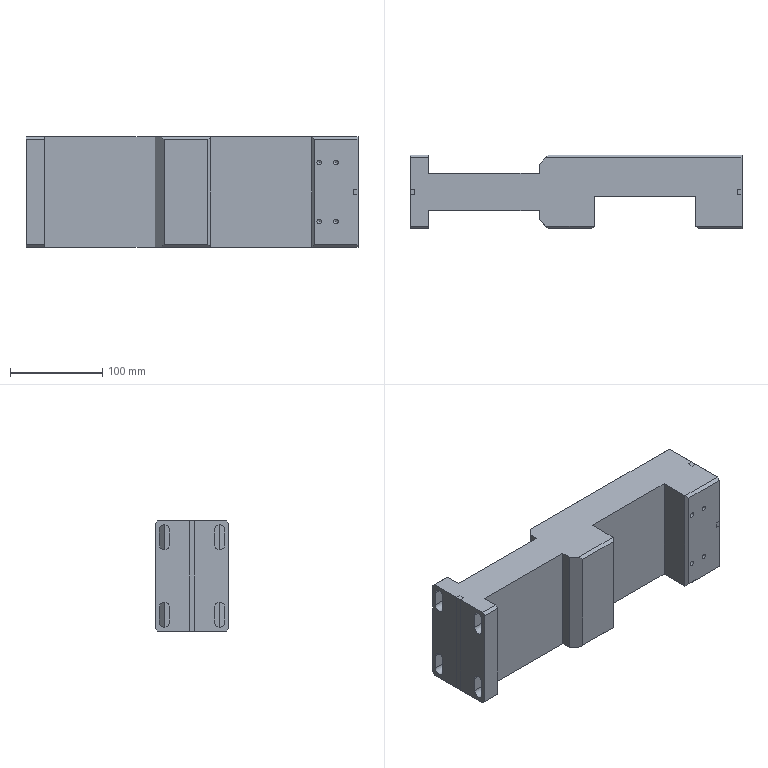CAM job | NX | 3+2 milling, drilling | part box 360 x 80 x 120 mm | stock box 365 x 85 x 125 mm
Tools:
number,name,description,diameter,corner_radius,flute_length,length,flutes
4,D4,平底铣刀-粗,4.0,0.0,25.0,75.0,2
6,D6,平底铣刀-粗,6.0,0.0,25.0,75.0,2
9,D10,平底铣刀-粗,10.0,0.0,35.0,75.0,2
23,D16,平底铣刀-粗,16.0,0.0,50.0,75.0,2
11,D4-J,平底铣刀-精,4.0,0.0,50.0,75.0,2
7,D6-J,平底铣刀-精,6.0,0.0,25.0,75.0,2
10,D10-J,平底铣刀-精,10.0,0.0,35.0,75.0,2
24,D16-J,平底铣刀-精,16.0,0.0,50.0,75.0,2
17,D6R0.5,圆鼻刀-粗,6.0,0.5,50.0,75.0,2
1,D80R0.8飞刀,圆鼻刀-粗,80.0,0.8,50.0,75.0,2
1,D80R0.8飞刀-J,圆鼻刀-精,80.0,0.8,50.0,75.0,2
2,D6倒角刀,倒角刀,6.0,0.0,3.0,25.0,2
18,M6X1.0,丝锥,5.0,0.0,35.0,50.0,2
17,M8X1.25,丝锥,6.8,0.0,35.0,50.0,2
15,ZT5.1,钻头,5.1,0.0,35.0,50.0,2
16,ZT6.9,Drilling Tool,6.9,0.0,35.0,50.0,2
Operations:
program,operation,operation_type,tool,method,geometry_group,spindle_rpm,surface_speed,feed_per_tooth,feed_cut,feed_plunge,cut_length_mm,path_length_mm,cut_time_min,machine_time_min
A,顶面,FaceMilling,D80R0.8飞刀,侧刃精光-切深K-步距G,W-A,4500.0,1385.0,0.1667,1500.0,100.0,1434.0,1530.0,0.956,0.9656
A,打点-深0.8,Operation,D6倒角刀,NONE,W-A,8000.0,150.796,0.0312,500.0,90.0,7.2,217.463,0.0144,0.0354
A,NG_盲锥孔-M6螺纹底孔,Operation,ZT5.1,NONE,W-A,2500.0,39.27,0.03,150.0,90.0,80.0,363.063,0.5333,0.5616
A,外形粗_2,VolumeBased25DMillingOperation,D16,METHOD,W-A,6000.0,301.593,0.5,6000.0,80.0,103112.699,103291.199,17.185,17.203
A,底壁粗_1,VolumeBased25DMillingOperation,D10,METHOD,W-A,9000.0,282.743,0.3333,6000.0,100.0,90760.242,93048.363,15.127,15.355
A,型腔铣开粗-中_COPY,CavityMilling,D10,分层开粗-切深K-步距G,W-A,8000.0,251.32,0.25,4000.0,100.0,7408.75,7808.48,1.852,1.907
A,型腔铣开粗-中_COPY_COPY,CavityMilling,D10,分层开粗-切深K-步距G,W-A,8000.0,251.32,0.25,4000.0,100.0,6245.453,7228.488,1.561,1.694
A,仅选体,SurfaceContour,D6倒角刀,METHOD,W-A,8000.0,150.796,0.1875,3000.0,100.0,673.495,1903.981,0.2245,0.3475
A,铣倒角_1,PlanarMilling,D6倒角刀,METHOD,W-A,8000.0,150.796,0.0375,600.0,100.0,75.821,582.245,0.1264,0.177
A,等高精光往复爬面_COPY,ZLevelMilling,D6R0.5,等高爬面-切深K-步距G,W-A,8000.0,150.796,0.25,4000.0,100.0,18105.798,18137.444,4.526,4.53
A,等高精光往复爬面_COPY_COPY,ZLevelMilling,D6R0.5,等高爬面-切深K-步距G,W-A,8000.0,150.796,0.25,4000.0,100.0,23657.928,24279.462,5.915,5.977
A,底精_1,VolumeBased25DMillingOperation,D10-J,METHOD,W-A,9000.0,169.646,0.0833,1500.0,100.0,2237.2,2376.2,1.492,1.505
A,底侧精_3,VolumeBased25DMillingOperation,D10-J,METHOD,W-A,9000.0,169.646,0.0833,1500.0,100.0,800.05,2139.41,0.5334,0.6673
A,盲锥孔-攻牙M6,Operation,M6X1.0,METHOD,W-A,500.0,7.854,0.001,1.0,90.0,64.0,331.063,64.0,64.027
A,外形半精_2,VolumeBased25DMillingOperation,D16-J,METHOD,W-A,5000.0,251.327,0.12,1200.0,100.0,7106.76,8454.822,5.922,6.057
B,底壁铣飞面开粗_COPY,VolumeBased25DMillingOperation,D80R0.8飞刀,分层开粗-切深K-步距G,W-B,2800.0,703.696,0.5357,3000.0,100.0,8697.187,9307.757,2.899,2.96
B,底壁铣飞面精光_COPY,VolumeBased25DMillingOperation,D80R0.8飞刀-J,侧刃精光-切深K-步距G,W-B,4000.0,1005.28,0.125,1000.0,100.0,1399.584,1495.584,1.4,1.409
B,型腔铣开粗-中_COPY_1,CavityMilling,D10,分层开粗-切深K-步距G,W-B,8000.0,251.32,0.25,4000.0,100.0,167817.825,175313.691,41.955,43.014
B,打点-深0.8_2,Operation,D6倒角刀,NONE,W-B,8000.0,150.796,0.0312,500.0,90.0,7.2,217.463,0.0144,0.0354
B,NG_盲锥孔-M6螺纹底孔_2,Operation,ZT5.1,NONE,W-B,2500.0,39.27,0.03,150.0,90.0,80.0,363.063,0.5333,0.5616
B,底壁铣精光底面-中_COPY,VolumeBased25DMillingOperation,D10-J,精光步距切深关,W-B,7000.0,175.0,0.0536,1500.0,100.0,5552.641,5907.622,3.702,3.737
B,等高精光往复爬面_COPY_COPY_1,ZLevelMilling,D6R0.5,等高爬面-切深K-步距G,W-B,8000.0,150.796,0.25,4000.0,100.0,18105.804,18144.874,4.527,4.53
B,等高精光往复爬面_COPY_COPY_1_COPY,ZLevelMilling,D6R0.5,等高爬面-切深K-步距G,W-B,8000.0,150.796,0.25,4000.0,100.0,30508.6,31097.257,7.627,7.686
B,平面去毛刺6X45L_COPY,SurfaceContour,D6倒角刀,爬面_倒角-切深0-步距G,W-B,6500.0,122.519,0.1154,1500.0,100.0,1027.274,2443.977,0.6848,0.8265
B,铣倒角_2,PlanarMilling,D6倒角刀,METHOD,W-B,8000.0,150.796,0.0375,600.0,100.0,75.821,582.245,0.1264,0.177
B,盲锥孔-攻牙M6_2,Operation,M6X1.0,METHOD,W-B,500.0,7.854,0.001,1.0,90.0,64.0,331.063,64.0,64.027
B,底壁铣精光侧面-中-选底面_COPY,VolumeBased25DMillingOperation,D10-J,侧刃精光-切深K-步距G,W-B,8000.0,251.32,0.0625,1000.0,100.0,554.724,929.003,0.5547,0.5922
B,底壁铣精光侧面-中-选底面_COPY_1,VolumeBased25DMillingOperation,D10-J,侧刃精光-切深K-步距G,W-B,8000.0,251.32,0.0625,1000.0,100.0,1109.451,1850.612,1.109,1.184
D,底壁铣螺旋开粗-中_COPY,VolumeBased25DMillingOperation,D6,分层开粗-切深K-步距G,W-D,8000.0,150.796,0.125,2000.0,100.0,8133.076,8800.416,4.066,4.133
D,底壁铣分层开粗-中_COPY_1,VolumeBased25DMillingOperation,D4,分层开粗-切深K-步距G,W-D,8000.0,100.528,0.125,2000.0,100.0,4528.8,4610.955,2.264,2.273
D,平面去毛刺6X45L_COPY_2,SurfaceContour,D6倒角刀,爬面_倒角-切深0-步距G,W-D,6500.0,122.519,0.1154,1500.0,100.0,896.525,1415.715,0.5977,0.6496
D,底壁铣螺旋精光-中_COPY,VolumeBased25DMillingOperation,D6-J,螺旋精光-切深K-步距G,W-D,8000.0,150.792,0.0625,1000.0,100.0,1193.037,1877.524,1.193,1.262
D,底壁铣精光侧面-中-选底面_COPY_3,VolumeBased25DMillingOperation,D4-J,侧刃精光-切深K-步距G,W-D,8000.0,100.528,0.05,800.0,100.0,255.552,283.553,0.3194,0.3222
C,打点-深0.8_3,Operation,D6倒角刀,NONE,W-C,8000.0,150.796,0.0312,500.0,90.0,7.2,337.422,0.0144,0.0474
C,NG_盲锥孔-M8螺纹底孔,Operation,ZT6.9,NONE,W-C,2200.0,46.998,0.0341,150.0,90.0,104.0,531.022,0.6933,0.736
C,铣倒角_3,PlanarMilling,D6倒角刀,METHOD,W-C,8000.0,150.796,0.0375,600.0,100.0,97.605,724.85,0.1627,0.2254
C,盲锥孔-攻牙M8,Operation,M8X1.25,METHOD,W-C,500.0,10.681,0.0013,1.25,90.0,81.0,485.022,64.8,64.84
C,底壁铣分层开粗-中_COPY,VolumeBased25DMillingOperation,D4,分层开粗-切深K-步距G,W-C,8000.0,100.528,0.125,2000.0,100.0,5956.44,5986.824,2.978,2.981
C,平面去毛刺6X45L_COPY_1,SurfaceContour,D6倒角刀,爬面_倒角-切深0-步距G,W-C,6500.0,122.519,0.1154,1500.0,100.0,860.257,1394.65,0.5735,0.6269
C,底壁铣精光侧面-中-选底面_COPY_2,VolumeBased25DMillingOperation,D4-J,侧刃精光-切深K-步距G,W-C,8000.0,100.531,0.0625,1000.0,100.0,421.329,449.332,0.4213,0.4241